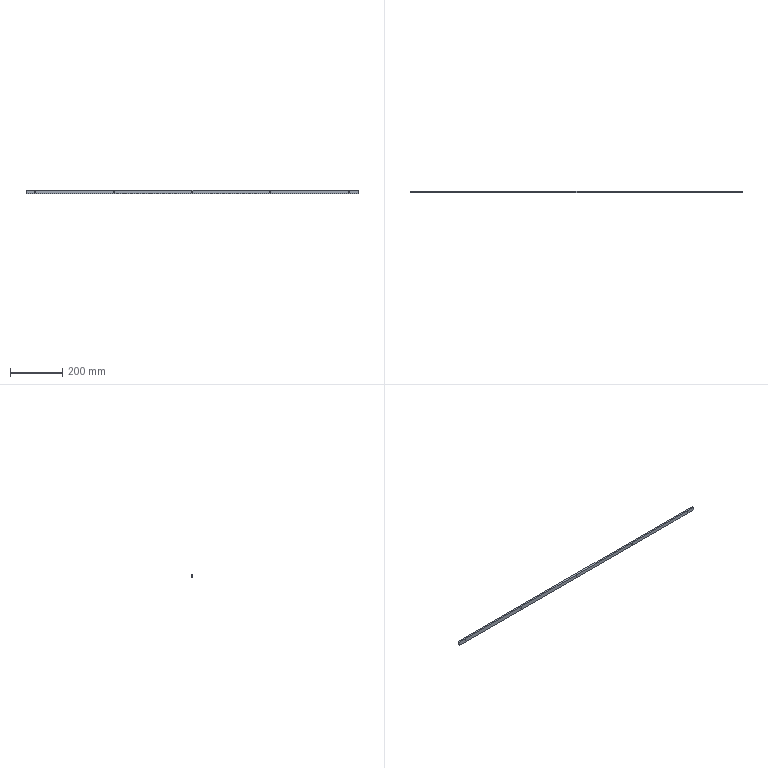Part | SolidWorks | features Chamfer 1, Extrusion 1, HoleWzd 1 | 1 solid | 33 faces | box 1270 x 6 x 15 mm | volume 113647 mm3 | cylinder 20 | plane 13 | commonest cylinder face diameters 3.4 x10 6 x10
STEP:
#1=CARTESIAN_POINT('',(-600.,-0.4,-3.));
#2=VERTEX_POINT('',#1);
#3=CARTESIAN_POINT('',(-600.,-0.4,3.));
#4=VERTEX_POINT('',#3);
#5=CARTESIAN_POINT('',(-600.,-0.4,0.));
#6=DIRECTION('',(0.,1.,0.));
#7=DIRECTION('',(0.,0.,1.));
#8=AXIS2_PLACEMENT_3D('',#5,#6,#7);
#9=CIRCLE('',#8,3.);
#10=EDGE_CURVE('',#2,#4,#9,.T.);
#11=ORIENTED_EDGE('',*,*,#10,.F.);
#12=CARTESIAN_POINT('',(-600.,3.,-3.));
#13=VERTEX_POINT('',#12);
#14=CARTESIAN_POINT('',(-600.,3.,-3.));
#15=DIRECTION('',(0.,1.,0.));
#16=VECTOR('',#15,1000.);
#17=LINE('',#14,#16);
#18=EDGE_CURVE('',#2,#13,#17,.T.);
#19=ORIENTED_EDGE('',*,*,#18,.T.);
#20=CARTESIAN_POINT('',(-600.,3.,3.));
#21=VERTEX_POINT('',#20);
#22=CARTESIAN_POINT('',(-600.,3.,0.));
#23=DIRECTION('',(0.,1.,0.));
#24=DIRECTION('',(0.,0.,1.));
#25=AXIS2_PLACEMENT_3D('',#22,#23,#24);
#26=CIRCLE('',#25,3.);
#27=EDGE_CURVE('',#13,#21,#26,.T.);
#28=ORIENTED_EDGE('',*,*,#27,.T.);
#29=CARTESIAN_POINT('',(-600.,3.,3.));
#30=DIRECTION('',(0.,1.,0.));
#31=VECTOR('',#30,1000.);
#32=LINE('',#29,#31);
#33=EDGE_CURVE('',#4,#21,#32,.T.);
#34=ORIENTED_EDGE('',*,*,#33,.F.);
#35=EDGE_LOOP('',(#11,#19,#28,#34));
#36=FACE_OUTER_BOUND('',#35,.T.);
#37=CARTESIAN_POINT('',(-600.,3.,0.));
#38=DIRECTION('',(0.,1.,0.));
#39=DIRECTION('',(0.,0.,1.));
#40=AXIS2_PLACEMENT_3D('',#37,#38,#39);
#41=CYLINDRICAL_SURFACE('',#40,3.);
#42=ADVANCED_FACE('',(#36),#41,.F.);
#43=CARTESIAN_POINT('',(-600.,-3.,-1.7));
#44=VERTEX_POINT('',#43);
#45=CARTESIAN_POINT('',(-600.,-3.,1.7));
#46=VERTEX_POINT('',#45);
#47=CARTESIAN_POINT('',(-600.,-3.,0.));
#48=DIRECTION('',(0.,1.,0.));
#49=DIRECTION('',(0.,0.,1.));
#50=AXIS2_PLACEMENT_3D('',#47,#48,#49);
#51=CIRCLE('',#50,1.7);
#52=EDGE_CURVE('',#44,#46,#51,.T.);
#53=ORIENTED_EDGE('',*,*,#52,.F.);
#54=CARTESIAN_POINT('',(-600.,-0.4,-1.7));
#55=VERTEX_POINT('',#54);
#56=CARTESIAN_POINT('',(-600.,3.,-1.7));
#57=DIRECTION('',(0.,1.,0.));
#58=VECTOR('',#57,1000.);
#59=LINE('',#56,#58);
#60=EDGE_CURVE('',#44,#55,#59,.T.);
#61=ORIENTED_EDGE('',*,*,#60,.T.);
#62=CARTESIAN_POINT('',(-600.,-0.4,1.7));
#63=VERTEX_POINT('',#62);
#64=CARTESIAN_POINT('',(-600.,-0.4,0.));
#65=DIRECTION('',(0.,1.,0.));
#66=DIRECTION('',(0.,0.,1.));
#67=AXIS2_PLACEMENT_3D('',#64,#65,#66);
#68=CIRCLE('',#67,1.7);
#69=EDGE_CURVE('',#55,#63,#68,.T.);
#70=ORIENTED_EDGE('',*,*,#69,.T.);
#71=CARTESIAN_POINT('',(-600.,3.,1.7));
#72=DIRECTION('',(0.,1.,0.));
#73=VECTOR('',#72,1000.);
#74=LINE('',#71,#73);
#75=EDGE_CURVE('',#46,#63,#74,.T.);
#76=ORIENTED_EDGE('',*,*,#75,.F.);
#77=EDGE_LOOP('',(#53,#61,#70,#76));
#78=FACE_OUTER_BOUND('',#77,.T.);
#79=CARTESIAN_POINT('',(-600.,3.,0.));
#80=DIRECTION('',(0.,1.,0.));
#81=DIRECTION('',(0.,0.,1.));
#82=AXIS2_PLACEMENT_3D('',#79,#80,#81);
#83=CYLINDRICAL_SURFACE('',#82,1.7);
#84=ADVANCED_FACE('',(#78),#83,.F.);
#85=CARTESIAN_POINT('',(-300.,-0.4,-3.));
#86=VERTEX_POINT('',#85);
#87=CARTESIAN_POINT('',(-300.,-0.4,3.));
#88=VERTEX_POINT('',#87);
#89=CARTESIAN_POINT('',(-300.,-0.4,0.));
#90=DIRECTION('',(0.,1.,0.));
#91=DIRECTION('',(0.,0.,1.));
#92=AXIS2_PLACEMENT_3D('',#89,#90,#91);
#93=CIRCLE('',#92,3.);
#94=EDGE_CURVE('',#86,#88,#93,.T.);
#95=ORIENTED_EDGE('',*,*,#94,.F.);
#96=CARTESIAN_POINT('',(-300.,3.,-3.));
#97=VERTEX_POINT('',#96);
#98=CARTESIAN_POINT('',(-300.,3.,-3.));
#99=DIRECTION('',(0.,1.,0.));
#100=VECTOR('',#99,1000.);
#101=LINE('',#98,#100);
#102=EDGE_CURVE('',#86,#97,#101,.T.);
#103=ORIENTED_EDGE('',*,*,#102,.T.);
#104=CARTESIAN_POINT('',(-300.,3.,3.));
#105=VERTEX_POINT('',#104);
#106=CARTESIAN_POINT('',(-300.,3.,0.));
#107=DIRECTION('',(0.,1.,0.));
#108=DIRECTION('',(0.,0.,1.));
#109=AXIS2_PLACEMENT_3D('',#106,#107,#108);
#110=CIRCLE('',#109,3.);
#111=EDGE_CURVE('',#97,#105,#110,.T.);
#112=ORIENTED_EDGE('',*,*,#111,.T.);
#113=CARTESIAN_POINT('',(-300.,3.,3.));
#114=DIRECTION('',(0.,1.,0.));
#115=VECTOR('',#114,1000.);
#116=LINE('',#113,#115);
#117=EDGE_CURVE('',#88,#105,#116,.T.);
#118=ORIENTED_EDGE('',*,*,#117,.F.);
#119=EDGE_LOOP('',(#95,#103,#112,#118));
#120=FACE_OUTER_BOUND('',#119,.T.);
#121=CARTESIAN_POINT('',(-300.,3.,0.));
#122=DIRECTION('',(0.,1.,0.));
#123=DIRECTION('',(0.,0.,1.));
#124=AXIS2_PLACEMENT_3D('',#121,#122,#123);
#125=CYLINDRICAL_SURFACE('',#124,3.);
#126=ADVANCED_FACE('',(#120),#125,.F.);
#127=CARTESIAN_POINT('',(-300.,-3.,-1.7));
#128=VERTEX_POINT('',#127);
#129=CARTESIAN_POINT('',(-300.,-3.,1.7));
#130=VERTEX_POINT('',#129);
#131=CARTESIAN_POINT('',(-300.,-3.,0.));
#132=DIRECTION('',(0.,1.,0.));
#133=DIRECTION('',(0.,0.,1.));
#134=AXIS2_PLACEMENT_3D('',#131,#132,#133);
#135=CIRCLE('',#134,1.7);
#136=EDGE_CURVE('',#128,#130,#135,.T.);
#137=ORIENTED_EDGE('',*,*,#136,.F.);
#138=CARTESIAN_POINT('',(-300.,-0.4,-1.7));
#139=VERTEX_POINT('',#138);
#140=CARTESIAN_POINT('',(-300.,3.,-1.7));
#141=DIRECTION('',(0.,1.,0.));
#142=VECTOR('',#141,1000.);
#143=LINE('',#140,#142);
#144=EDGE_CURVE('',#128,#139,#143,.T.);
#145=ORIENTED_EDGE('',*,*,#144,.T.);
#146=CARTESIAN_POINT('',(-300.,-0.4,1.7));
#147=VERTEX_POINT('',#146);
#148=CARTESIAN_POINT('',(-300.,-0.4,0.));
#149=DIRECTION('',(0.,1.,0.));
#150=DIRECTION('',(0.,0.,1.));
#151=AXIS2_PLACEMENT_3D('',#148,#149,#150);
#152=CIRCLE('',#151,1.7);
#153=EDGE_CURVE('',#139,#147,#152,.T.);
#154=ORIENTED_EDGE('',*,*,#153,.T.);
#155=CARTESIAN_POINT('',(-300.,3.,1.7));
#156=DIRECTION('',(0.,1.,0.));
#157=VECTOR('',#156,1000.);
#158=LINE('',#155,#157);
#159=EDGE_CURVE('',#130,#147,#158,.T.);
#160=ORIENTED_EDGE('',*,*,#159,.F.);
#161=EDGE_LOOP('',(#137,#145,#154,#160));
#162=FACE_OUTER_BOUND('',#161,.T.);
#163=CARTESIAN_POINT('',(-300.,3.,0.));
#164=DIRECTION('',(0.,1.,0.));
#165=DIRECTION('',(0.,0.,1.));
#166=AXIS2_PLACEMENT_3D('',#163,#164,#165);
#167=CYLINDRICAL_SURFACE('',#166,1.7);
#168=ADVANCED_FACE('',(#162),#167,.F.);
#169=CARTESIAN_POINT('',(0.,-0.4,-3.));
#170=VERTEX_POINT('',#169);
#171=CARTESIAN_POINT('',(0.,-0.4,3.));
#172=VERTEX_POINT('',#171);
#173=CARTESIAN_POINT('',(0.,-0.4,0.));
#174=DIRECTION('',(0.,1.,0.));
#175=DIRECTION('',(0.,0.,1.));
#176=AXIS2_PLACEMENT_3D('',#173,#174,#175);
#177=CIRCLE('',#176,3.);
#178=EDGE_CURVE('',#170,#172,#177,.T.);
#179=ORIENTED_EDGE('',*,*,#178,.F.);
#180=CARTESIAN_POINT('',(0.,3.,-3.));
#181=VERTEX_POINT('',#180);
#182=CARTESIAN_POINT('',(0.,3.,-3.));
#183=DIRECTION('',(0.,1.,0.));
#184=VECTOR('',#183,1000.);
#185=LINE('',#182,#184);
#186=EDGE_CURVE('',#170,#181,#185,.T.);
#187=ORIENTED_EDGE('',*,*,#186,.T.);
#188=CARTESIAN_POINT('',(0.,3.,3.));
#189=VERTEX_POINT('',#188);
#190=CARTESIAN_POINT('',(0.,3.,0.));
#191=DIRECTION('',(0.,1.,0.));
#192=DIRECTION('',(0.,0.,1.));
#193=AXIS2_PLACEMENT_3D('',#190,#191,#192);
#194=CIRCLE('',#193,3.);
#195=EDGE_CURVE('',#181,#189,#194,.T.);
#196=ORIENTED_EDGE('',*,*,#195,.T.);
#197=CARTESIAN_POINT('',(0.,3.,3.));
#198=DIRECTION('',(0.,1.,0.));
#199=VECTOR('',#198,1000.);
#200=LINE('',#197,#199);
#201=EDGE_CURVE('',#172,#189,#200,.T.);
#202=ORIENTED_EDGE('',*,*,#201,.F.);
#203=EDGE_LOOP('',(#179,#187,#196,#202));
#204=FACE_OUTER_BOUND('',#203,.T.);
#205=CARTESIAN_POINT('',(0.,3.,0.));
#206=DIRECTION('',(0.,1.,0.));
#207=DIRECTION('',(0.,0.,1.));
#208=AXIS2_PLACEMENT_3D('',#205,#206,#207);
#209=CYLINDRICAL_SURFACE('',#208,3.);
#210=ADVANCED_FACE('',(#204),#209,.F.);
#211=CARTESIAN_POINT('',(0.,-3.,-1.7));
#212=VERTEX_POINT('',#211);
#213=CARTESIAN_POINT('',(0.,-3.,1.7));
#214=VERTEX_POINT('',#213);
#215=CARTESIAN_POINT('',(0.,-3.,0.));
#216=DIRECTION('',(0.,1.,0.));
#217=DIRECTION('',(0.,0.,1.));
#218=AXIS2_PLACEMENT_3D('',#215,#216,#217);
#219=CIRCLE('',#218,1.7);
#220=EDGE_CURVE('',#212,#214,#219,.T.);
#221=ORIENTED_EDGE('',*,*,#220,.F.);
#222=CARTESIAN_POINT('',(0.,-0.4,-1.7));
#223=VERTEX_POINT('',#222);
#224=CARTESIAN_POINT('',(0.,3.,-1.7));
#225=DIRECTION('',(0.,1.,0.));
#226=VECTOR('',#225,1000.);
#227=LINE('',#224,#226);
#228=EDGE_CURVE('',#212,#223,#227,.T.);
#229=ORIENTED_EDGE('',*,*,#228,.T.);
#230=CARTESIAN_POINT('',(0.,-0.4,1.7));
#231=VERTEX_POINT('',#230);
#232=CARTESIAN_POINT('',(0.,-0.4,0.));
#233=DIRECTION('',(0.,1.,0.));
#234=DIRECTION('',(0.,0.,1.));
#235=AXIS2_PLACEMENT_3D('',#232,#233,#234);
#236=CIRCLE('',#235,1.7);
#237=EDGE_CURVE('',#223,#231,#236,.T.);
#238=ORIENTED_EDGE('',*,*,#237,.T.);
#239=CARTESIAN_POINT('',(0.,3.,1.7));
#240=DIRECTION('',(0.,1.,0.));
#241=VECTOR('',#240,1000.);
#242=LINE('',#239,#241);
#243=EDGE_CURVE('',#214,#231,#242,.T.);
#244=ORIENTED_EDGE('',*,*,#243,.F.);
#245=EDGE_LOOP('',(#221,#229,#238,#244));
#246=FACE_OUTER_BOUND('',#245,.T.);
#247=CARTESIAN_POINT('',(0.,3.,0.));
#248=DIRECTION('',(0.,1.,0.));
#249=DIRECTION('',(0.,0.,1.));
#250=AXIS2_PLACEMENT_3D('',#247,#248,#249);
#251=CYLINDRICAL_SURFACE('',#250,1.7);
#252=ADVANCED_FACE('',(#246),#251,.F.);
#253=CARTESIAN_POINT('',(300.,-0.4,-3.));
#254=VERTEX_POINT('',#253);
#255=CARTESIAN_POINT('',(300.,-0.4,3.));
#256=VERTEX_POINT('',#255);
#257=CARTESIAN_POINT('',(300.,-0.4,0.));
#258=DIRECTION('',(0.,1.,0.));
#259=DIRECTION('',(0.,0.,1.));
#260=AXIS2_PLACEMENT_3D('',#257,#258,#259);
#261=CIRCLE('',#260,3.);
#262=EDGE_CURVE('',#254,#256,#261,.T.);
#263=ORIENTED_EDGE('',*,*,#262,.F.);
#264=CARTESIAN_POINT('',(300.,3.,-3.));
#265=VERTEX_POINT('',#264);
#266=CARTESIAN_POINT('',(300.,3.,-3.));
#267=DIRECTION('',(0.,1.,0.));
#268=VECTOR('',#267,1000.);
#269=LINE('',#266,#268);
#270=EDGE_CURVE('',#254,#265,#269,.T.);
#271=ORIENTED_EDGE('',*,*,#270,.T.);
#272=CARTESIAN_POINT('',(300.,3.,3.));
#273=VERTEX_POINT('',#272);
#274=CARTESIAN_POINT('',(300.,3.,0.));
#275=DIRECTION('',(0.,1.,0.));
#276=DIRECTION('',(0.,0.,1.));
#277=AXIS2_PLACEMENT_3D('',#274,#275,#276);
#278=CIRCLE('',#277,3.);
#279=EDGE_CURVE('',#265,#273,#278,.T.);
#280=ORIENTED_EDGE('',*,*,#279,.T.);
#281=CARTESIAN_POINT('',(300.,3.,3.));
#282=DIRECTION('',(0.,1.,0.));
#283=VECTOR('',#282,1000.);
#284=LINE('',#281,#283);
#285=EDGE_CURVE('',#256,#273,#284,.T.);
#286=ORIENTED_EDGE('',*,*,#285,.F.);
#287=EDGE_LOOP('',(#263,#271,#280,#286));
#288=FACE_OUTER_BOUND('',#287,.T.);
#289=CARTESIAN_POINT('',(300.,3.,0.));
#290=DIRECTION('',(0.,1.,0.));
#291=DIRECTION('',(0.,0.,1.));
#292=AXIS2_PLACEMENT_3D('',#289,#290,#291);
#293=CYLINDRICAL_SURFACE('',#292,3.);
#294=ADVANCED_FACE('',(#288),#293,.F.);
#295=CARTESIAN_POINT('',(300.,-3.,-1.7));
#296=VERTEX_POINT('',#295);
#297=CARTESIAN_POINT('',(300.,-3.,1.7));
#298=VERTEX_POINT('',#297);
#299=CARTESIAN_POINT('',(300.,-3.,0.));
#300=DIRECTION('',(0.,1.,0.));
#301=DIRECTION('',(0.,0.,1.));
#302=AXIS2_PLACEMENT_3D('',#299,#300,#301);
#303=CIRCLE('',#302,1.7);
#304=EDGE_CURVE('',#296,#298,#303,.T.);
#305=ORIENTED_EDGE('',*,*,#304,.F.);
#306=CARTESIAN_POINT('',(300.,-0.4,-1.7));
#307=VERTEX_POINT('',#306);
#308=CARTESIAN_POINT('',(300.,3.,-1.7));
#309=DIRECTION('',(0.,1.,0.));
#310=VECTOR('',#309,1000.);
#311=LINE('',#308,#310);
#312=EDGE_CURVE('',#296,#307,#311,.T.);
#313=ORIENTED_EDGE('',*,*,#312,.T.);
#314=CARTESIAN_POINT('',(300.,-0.4,1.7));
#315=VERTEX_POINT('',#314);
#316=CARTESIAN_POINT('',(300.,-0.4,0.));
#317=DIRECTION('',(0.,1.,0.));
#318=DIRECTION('',(0.,0.,1.));
#319=AXIS2_PLACEMENT_3D('',#316,#317,#318);
#320=CIRCLE('',#319,1.7);
#321=EDGE_CURVE('',#307,#315,#320,.T.);
#322=ORIENTED_EDGE('',*,*,#321,.T.);
#323=CARTESIAN_POINT('',(300.,3.,1.7));
#324=DIRECTION('',(0.,1.,0.));
#325=VECTOR('',#324,1000.);
#326=LINE('',#323,#325);
#327=EDGE_CURVE('',#298,#315,#326,.T.);
#328=ORIENTED_EDGE('',*,*,#327,.F.);
#329=EDGE_LOOP('',(#305,#313,#322,#328));
#330=FACE_OUTER_BOUND('',#329,.T.);
#331=CARTESIAN_POINT('',(300.,3.,0.));
#332=DIRECTION('',(0.,1.,0.));
#333=DIRECTION('',(0.,0.,1.));
#334=AXIS2_PLACEMENT_3D('',#331,#332,#333);
#335=CYLINDRICAL_SURFACE('',#334,1.7);
#336=ADVANCED_FACE('',(#330),#335,.F.);
#337=CARTESIAN_POINT('',(600.,-0.4,-3.));
#338=VERTEX_POINT('',#337);
#339=CARTESIAN_POINT('',(600.,-0.4,3.));
#340=VERTEX_POINT('',#339);
#341=CARTESIAN_POINT('',(600.,-0.4,0.));
#342=DIRECTION('',(0.,1.,0.));
#343=DIRECTION('',(0.,0.,1.));
#344=AXIS2_PLACEMENT_3D('',#341,#342,#343);
#345=CIRCLE('',#344,3.);
#346=EDGE_CURVE('',#338,#340,#345,.T.);
#347=ORIENTED_EDGE('',*,*,#346,.F.);
#348=CARTESIAN_POINT('',(600.,3.,-3.));
#349=VERTEX_POINT('',#348);
#350=CARTESIAN_POINT('',(600.,3.,-3.));
#351=DIRECTION('',(0.,1.,0.));
#352=VECTOR('',#351,1000.);
#353=LINE('',#350,#352);
#354=EDGE_CURVE('',#338,#349,#353,.T.);
#355=ORIENTED_EDGE('',*,*,#354,.T.);
#356=CARTESIAN_POINT('',(600.,3.,3.));
#357=VERTEX_POINT('',#356);
#358=CARTESIAN_POINT('',(600.,3.,0.));
#359=DIRECTION('',(0.,1.,0.));
#360=DIRECTION('',(0.,0.,1.));
#361=AXIS2_PLACEMENT_3D('',#358,#359,#360);
#362=CIRCLE('',#361,3.);
#363=EDGE_CURVE('',#349,#357,#362,.T.);
#364=ORIENTED_EDGE('',*,*,#363,.T.);
#365=CARTESIAN_POINT('',(600.,3.,3.));
#366=DIRECTION('',(0.,1.,0.));
#367=VECTOR('',#366,1000.);
#368=LINE('',#365,#367);
#369=EDGE_CURVE('',#340,#357,#368,.T.);
#370=ORIENTED_EDGE('',*,*,#369,.F.);
#371=EDGE_LOOP('',(#347,#355,#364,#370));
#372=FACE_OUTER_BOUND('',#371,.T.);
#373=CARTESIAN_POINT('',(600.,3.,0.));
#374=DIRECTION('',(0.,1.,0.));
#375=DIRECTION('',(0.,0.,1.));
#376=AXIS2_PLACEMENT_3D('',#373,#374,#375);
#377=CYLINDRICAL_SURFACE('',#376,3.);
#378=ADVANCED_FACE('',(#372),#377,.F.);
#379=CARTESIAN_POINT('',(600.,-3.,-1.7));
#380=VERTEX_POINT('',#379);
#381=CARTESIAN_POINT('',(600.,-3.,1.7));
#382=VERTEX_POINT('',#381);
#383=CARTESIAN_POINT('',(600.,-3.,0.));
#384=DIRECTION('',(0.,1.,0.));
#385=DIRECTION('',(0.,0.,1.));
#386=AXIS2_PLACEMENT_3D('',#383,#384,#385);
#387=CIRCLE('',#386,1.7);
#388=EDGE_CURVE('',#380,#382,#387,.T.);
#389=ORIENTED_EDGE('',*,*,#388,.F.);
#390=CARTESIAN_POINT('',(600.,-0.4,-1.7));
#391=VERTEX_POINT('',#390);
#392=CARTESIAN_POINT('',(600.,3.,-1.7));
#393=DIRECTION('',(0.,1.,0.));
#394=VECTOR('',#393,1000.);
#395=LINE('',#392,#394);
#396=EDGE_CURVE('',#380,#391,#395,.T.);
#397=ORIENTED_EDGE('',*,*,#396,.T.);
#398=CARTESIAN_POINT('',(600.,-0.4,1.7));
#399=VERTEX_POINT('',#398);
#400=CARTESIAN_POINT('',(600.,-0.4,0.));
#401=DIRECTION('',(0.,1.,0.));
#402=DIRECTION('',(0.,0.,1.));
#403=AXIS2_PLACEMENT_3D('',#400,#401,#402);
#404=CIRCLE('',#403,1.7);
#405=EDGE_CURVE('',#391,#399,#404,.T.);
#406=ORIENTED_EDGE('',*,*,#405,.T.);
#407=CARTESIAN_POINT('',(600.,3.,1.7));
#408=DIRECTION('',(0.,1.,0.));
#409=VECTOR('',#408,1000.);
#410=LINE('',#407,#409);
#411=EDGE_CURVE('',#382,#399,#410,.T.);
#412=ORIENTED_EDGE('',*,*,#411,.F.);
#413=EDGE_LOOP('',(#389,#397,#406,#412));
#414=FACE_OUTER_BOUND('',#413,.T.);
#415=CARTESIAN_POINT('',(600.,3.,0.));
#416=DIRECTION('',(0.,1.,0.));
#417=DIRECTION('',(0.,0.,1.));
#418=AXIS2_PLACEMENT_3D('',#415,#416,#417);
#419=CYLINDRICAL_SURFACE('',#418,1.7);
#420=ADVANCED_FACE('',(#414),#419,.F.);
#421=CARTESIAN_POINT('',(635.,3.,4.5));
#422=VERTEX_POINT('',#421);
#423=CARTESIAN_POINT('',(635.,3.,-7.5));
#424=VERTEX_POINT('',#423);
#425=CARTESIAN_POINT('',(635.,3.,7.5));
#426=DIRECTION('',(0.,0.,-1.));
#427=VECTOR('',#426,1000.);
#428=LINE('',#425,#427);
#429=EDGE_CURVE('',#422,#424,#428,.T.);
#430=ORIENTED_EDGE('',*,*,#429,.F.);
#431=CARTESIAN_POINT('',(635.,-3.,4.5));
#432=VERTEX_POINT('',#431);
#433=CARTESIAN_POINT('',(635.,3.,4.5));
#434=DIRECTION('',(0.,-1.,0.));
#435=VECTOR('',#434,1000.);
#436=LINE('',#433,#435);
#437=EDGE_CURVE('',#422,#432,#436,.T.);
#438=ORIENTED_EDGE('',*,*,#437,.T.);
#439=CARTESIAN_POINT('',(635.,-3.,-7.5));
#440=VERTEX_POINT('',#439);
#441=CARTESIAN_POINT('',(635.,-3.,7.5));
#442=DIRECTION('',(0.,0.,-1.));
#443=VECTOR('',#442,1000.);
#444=LINE('',#441,#443);
#445=EDGE_CURVE('',#432,#440,#444,.T.);
#446=ORIENTED_EDGE('',*,*,#445,.T.);
#447=CARTESIAN_POINT('',(635.,3.,-7.5));
#448=DIRECTION('',(0.,-1.,0.));
#449=VECTOR('',#448,1000.);
#450=LINE('',#447,#449);
#451=EDGE_CURVE('',#424,#440,#450,.T.);
#452=ORIENTED_EDGE('',*,*,#451,.F.);
#453=EDGE_LOOP('',(#430,#438,#446,#452));
#454=FACE_OUTER_BOUND('',#453,.T.);
#455=CARTESIAN_POINT('',(635.,3.,7.5));
#456=DIRECTION('',(-1.,0.,0.));
#457=DIRECTION('',(0.,0.,1.));
#458=AXIS2_PLACEMENT_3D('',#455,#456,#457);
#459=PLANE('',#458);
#460=ADVANCED_FACE('',(#454),#459,.F.);
#461=CARTESIAN_POINT('',(-635.,-3.,-7.5));
#462=VERTEX_POINT('',#461);
#463=CARTESIAN_POINT('',(-635.,-3.,-7.5));
#464=DIRECTION('',(-1.,0.,0.));
#465=VECTOR('',#464,1000.);
#466=LINE('',#463,#465);
#467=EDGE_CURVE('',#440,#462,#466,.T.);
#468=ORIENTED_EDGE('',*,*,#467,.T.);
#469=CARTESIAN_POINT('',(-635.,3.,-7.5));
#470=VERTEX_POINT('',#469);
#471=CARTESIAN_POINT('',(-635.,3.,-7.5));
#472=DIRECTION('',(0.,-1.,0.));
#473=VECTOR('',#472,1000.);
#474=LINE('',#471,#473);
#475=EDGE_CURVE('',#470,#462,#474,.T.);
#476=ORIENTED_EDGE('',*,*,#475,.F.);
#477=CARTESIAN_POINT('',(-635.,3.,-7.5));
#478=DIRECTION('',(-1.,0.,0.));
#479=VECTOR('',#478,1000.);
#480=LINE('',#477,#479);
#481=EDGE_CURVE('',#424,#470,#480,.T.);
#482=ORIENTED_EDGE('',*,*,#481,.F.);
#483=ORIENTED_EDGE('',*,*,#451,.T.);
#484=EDGE_LOOP('',(#468,#476,#482,#483));
#485=FACE_OUTER_BOUND('',#484,.T.);
#486=CARTESIAN_POINT('',(-635.,3.,-7.5));
#487=DIRECTION('',(0.,0.,1.));
#488=DIRECTION('',(1.,0.,0.));
#489=AXIS2_PLACEMENT_3D('',#486,#487,#488);
#490=PLANE('',#489);
#491=ADVANCED_FACE('',(#485),#490,.F.);
#492=CARTESIAN_POINT('',(-635.,-3.,4.5));
#493=VERTEX_POINT('',#492);
#494=CARTESIAN_POINT('',(-635.,-3.,7.5));
#495=DIRECTION('',(0.,0.,1.));
#496=VECTOR('',#495,1000.);
#497=LINE('',#494,#496);
#498=EDGE_CURVE('',#462,#493,#497,.T.);
#499=ORIENTED_EDGE('',*,*,#498,.T.);
#500=CARTESIAN_POINT('',(-635.,3.,4.5));
#501=VERTEX_POINT('',#500);
#502=CARTESIAN_POINT('',(-635.,3.,4.5));
#503=DIRECTION('',(0.,1.,0.));
#504=VECTOR('',#503,1000.);
#505=LINE('',#502,#504);
#506=EDGE_CURVE('',#493,#501,#505,.T.);
#507=ORIENTED_EDGE('',*,*,#506,.T.);
#508=CARTESIAN_POINT('',(-635.,3.,7.5));
#509=DIRECTION('',(0.,0.,1.));
#510=VECTOR('',#509,1000.);
#511=LINE('',#508,#510);
#512=EDGE_CURVE('',#470,#501,#511,.T.);
#513=ORIENTED_EDGE('',*,*,#512,.F.);
#514=ORIENTED_EDGE('',*,*,#475,.T.);
#515=EDGE_LOOP('',(#499,#507,#513,#514));
#516=FACE_OUTER_BOUND('',#515,.T.);
#517=CARTESIAN_POINT('',(-635.,3.,7.5));
#518=DIRECTION('',(1.,0.,0.));
#519=DIRECTION('',(0.,0.,-1.));
#520=AXIS2_PLACEMENT_3D('',#517,#518,#519);
#521=PLANE('',#520);
#522=ADVANCED_FACE('',(#516),#521,.F.);
#523=CARTESIAN_POINT('',(-632.,3.,7.5));
#524=VERTEX_POINT('',#523);
#525=CARTESIAN_POINT('',(632.,3.,7.5));
#526=VERTEX_POINT('',#525);
#527=CARTESIAN_POINT('',(-635.,3.,7.5));
#528=DIRECTION('',(1.,0.,0.));
#529=VECTOR('',#528,1000.);
#530=LINE('',#527,#529);
#531=EDGE_CURVE('',#524,#526,#530,.T.);
#532=ORIENTED_EDGE('',*,*,#531,.F.);
#533=CARTESIAN_POINT('',(-632.,-3.,7.5));
#534=VERTEX_POINT('',#533);
#535=CARTESIAN_POINT('',(-632.,3.,7.5));
#536=DIRECTION('',(0.,-1.,0.));
#537=VECTOR('',#536,1000.);
#538=LINE('',#535,#537);
#539=EDGE_CURVE('',#524,#534,#538,.T.);
#540=ORIENTED_EDGE('',*,*,#539,.T.);
#541=CARTESIAN_POINT('',(632.,-3.,7.5));
#542=VERTEX_POINT('',#541);
#543=CARTESIAN_POINT('',(-635.,-3.,7.5));
#544=DIRECTION('',(1.,0.,0.));
#545=VECTOR('',#544,1000.);
#546=LINE('',#543,#545);
#547=EDGE_CURVE('',#534,#542,#546,.T.);
#548=ORIENTED_EDGE('',*,*,#547,.T.);
#549=CARTESIAN_POINT('',(632.,3.,7.5));
#550=DIRECTION('',(0.,1.,0.));
#551=VECTOR('',#550,1000.);
#552=LINE('',#549,#551);
#553=EDGE_CURVE('',#542,#526,#552,.T.);
#554=ORIENTED_EDGE('',*,*,#553,.T.);
#555=EDGE_LOOP('',(#532,#540,#548,#554));
#556=FACE_OUTER_BOUND('',#555,.T.);
#557=CARTESIAN_POINT('',(-635.,3.,7.5));
#558=DIRECTION('',(0.,0.,-1.));
#559=DIRECTION('',(-1.,0.,0.));
#560=AXIS2_PLACEMENT_3D('',#557,#558,#559);
#561=PLANE('',#560);
#562=ADVANCED_FACE('',(#556),#561,.F.);
#563=CARTESIAN_POINT('',(-600.,3.,0.));
#564=DIRECTION('',(0.,1.,0.));
#565=DIRECTION('',(0.,0.,1.));
#566=AXIS2_PLACEMENT_3D('',#563,#564,#565);
#567=CIRCLE('',#566,3.);
#568=EDGE_CURVE('',#21,#13,#567,.T.);
#569=ORIENTED_EDGE('',*,*,#568,.F.);
#570=ORIENTED_EDGE('',*,*,#27,.F.);
#571=EDGE_LOOP('',(#569,#570));
#572=FACE_BOUND('',#571,.T.);
#573=CARTESIAN_POINT('',(-300.,3.,0.));
#574=DIRECTION('',(0.,1.,0.));
#575=DIRECTION('',(0.,0.,1.));
#576=AXIS2_PLACEMENT_3D('',#573,#574,#575);
#577=CIRCLE('',#576,3.);
#578=EDGE_CURVE('',#105,#97,#577,.T.);
#579=ORIENTED_EDGE('',*,*,#578,.F.);
#580=ORIENTED_EDGE('',*,*,#111,.F.);
#581=EDGE_LOOP('',(#579,#580));
#582=FACE_BOUND('',#581,.T.);
#583=CARTESIAN_POINT('',(0.,3.,0.));
#584=DIRECTION('',(0.,1.,0.));
#585=DIRECTION('',(0.,0.,1.));
#586=AXIS2_PLACEMENT_3D('',#583,#584,#585);
#587=CIRCLE('',#586,3.);
#588=EDGE_CURVE('',#189,#181,#587,.T.);
#589=ORIENTED_EDGE('',*,*,#588,.F.);
#590=ORIENTED_EDGE('',*,*,#195,.F.);
#591=EDGE_LOOP('',(#589,#590));
#592=FACE_BOUND('',#591,.T.);
#593=CARTESIAN_POINT('',(300.,3.,0.));
#594=DIRECTION('',(0.,1.,0.));
#595=DIRECTION('',(0.,0.,1.));
#596=AXIS2_PLACEMENT_3D('',#593,#594,#595);
#597=CIRCLE('',#596,3.);
#598=EDGE_CURVE('',#273,#265,#597,.T.);
#599=ORIENTED_EDGE('',*,*,#598,.F.);
#600=ORIENTED_EDGE('',*,*,#279,.F.);
#601=EDGE_LOOP('',(#599,#600));
#602=FACE_BOUND('',#601,.T.);
#603=CARTESIAN_POINT('',(600.,3.,0.));
#604=DIRECTION('',(0.,1.,0.));
#605=DIRECTION('',(0.,0.,1.));
#606=AXIS2_PLACEMENT_3D('',#603,#604,#605);
#607=CIRCLE('',#606,3.);
#608=EDGE_CURVE('',#357,#349,#607,.T.);
#609=ORIENTED_EDGE('',*,*,#608,.F.);
#610=ORIENTED_EDGE('',*,*,#363,.F.);
#611=EDGE_LOOP('',(#609,#610));
#612=FACE_BOUND('',#611,.T.);
#613=ORIENTED_EDGE('',*,*,#512,.T.);
#614=CARTESIAN_POINT('',(-632.,3.,7.5));
#615=DIRECTION('',(0.7071,0.,0.7071));
#616=VECTOR('',#615,1000.);
#617=LINE('',#614,#616);
#618=EDGE_CURVE('',#501,#524,#617,.T.);
#619=ORIENTED_EDGE('',*,*,#618,.T.);
#620=ORIENTED_EDGE('',*,*,#531,.T.);
#621=CARTESIAN_POINT('',(635.,3.,4.5));
#622=DIRECTION('',(0.7071,0.,-0.7071));
#623=VECTOR('',#622,1000.);
#624=LINE('',#621,#623);
#625=EDGE_CURVE('',#526,#422,#624,.T.);
#626=ORIENTED_EDGE('',*,*,#625,.T.);
#627=ORIENTED_EDGE('',*,*,#429,.T.);
#628=ORIENTED_EDGE('',*,*,#481,.T.);
#629=EDGE_LOOP('',(#613,#619,#620,#626,#627,#628));
#630=FACE_OUTER_BOUND('',#629,.T.);
#631=CARTESIAN_POINT('',(0.,3.,0.));
#632=DIRECTION('',(0.,-1.,0.));
#633=DIRECTION('',(0.,0.,-1.));
#634=AXIS2_PLACEMENT_3D('',#631,#632,#633);
#635=PLANE('',#634);
#636=ADVANCED_FACE('',(#572,#582,#592,#602,#612,#630),#635,.F.);
#637=CARTESIAN_POINT('',(-600.,-3.,0.));
#638=DIRECTION('',(0.,1.,0.));
#639=DIRECTION('',(0.,0.,1.));
#640=AXIS2_PLACEMENT_3D('',#637,#638,#639);
#641=CIRCLE('',#640,1.7);
#642=EDGE_CURVE('',#46,#44,#641,.T.);
#643=ORIENTED_EDGE('',*,*,#642,.T.);
#644=ORIENTED_EDGE('',*,*,#52,.T.);
#645=EDGE_LOOP('',(#643,#644));
#646=FACE_BOUND('',#645,.T.);
#647=CARTESIAN_POINT('',(-300.,-3.,0.));
#648=DIRECTION('',(0.,1.,0.));
#649=DIRECTION('',(0.,0.,1.));
#650=AXIS2_PLACEMENT_3D('',#647,#648,#649);
#651=CIRCLE('',#650,1.7);
#652=EDGE_CURVE('',#130,#128,#651,.T.);
#653=ORIENTED_EDGE('',*,*,#652,.T.);
#654=ORIENTED_EDGE('',*,*,#136,.T.);
#655=EDGE_LOOP('',(#653,#654));
#656=FACE_BOUND('',#655,.T.);
#657=CARTESIAN_POINT('',(0.,-3.,0.));
#658=DIRECTION('',(0.,1.,0.));
#659=DIRECTION('',(0.,0.,1.));
#660=AXIS2_PLACEMENT_3D('',#657,#658,#659);
#661=CIRCLE('',#660,1.7);
#662=EDGE_CURVE('',#214,#212,#661,.T.);
#663=ORIENTED_EDGE('',*,*,#662,.T.);
#664=ORIENTED_EDGE('',*,*,#220,.T.);
#665=EDGE_LOOP('',(#663,#664));
#666=FACE_BOUND('',#665,.T.);
#667=CARTESIAN_POINT('',(300.,-3.,0.));
#668=DIRECTION('',(0.,1.,0.));
#669=DIRECTION('',(0.,0.,1.));
#670=AXIS2_PLACEMENT_3D('',#667,#668,#669);
#671=CIRCLE('',#670,1.7);
#672=EDGE_CURVE('',#298,#296,#671,.T.);
#673=ORIENTED_EDGE('',*,*,#672,.T.);
#674=ORIENTED_EDGE('',*,*,#304,.T.);
#675=EDGE_LOOP('',(#673,#674));
#676=FACE_BOUND('',#675,.T.);
#677=CARTESIAN_POINT('',(600.,-3.,0.));
#678=DIRECTION('',(0.,1.,0.));
#679=DIRECTION('',(0.,0.,1.));
#680=AXIS2_PLACEMENT_3D('',#677,#678,#679);
#681=CIRCLE('',#680,1.7);
#682=EDGE_CURVE('',#382,#380,#681,.T.);
#683=ORIENTED_EDGE('',*,*,#682,.T.);
#684=ORIENTED_EDGE('',*,*,#388,.T.);
#685=EDGE_LOOP('',(#683,#684));
#686=FACE_BOUND('',#685,.T.);
#687=ORIENTED_EDGE('',*,*,#547,.F.);
#688=CARTESIAN_POINT('',(-319.75,-3.,319.75));
#689=DIRECTION('',(-0.7071,0.,-0.7071));
#690=VECTOR('',#689,1000.);
#691=LINE('',#688,#690);
#692=EDGE_CURVE('',#534,#493,#691,.T.);
#693=ORIENTED_EDGE('',*,*,#692,.T.);
#694=ORIENTED_EDGE('',*,*,#498,.F.);
#695=ORIENTED_EDGE('',*,*,#467,.F.);
#696=ORIENTED_EDGE('',*,*,#445,.F.);
#697=CARTESIAN_POINT('',(319.75,-3.,319.75));
#698=DIRECTION('',(-0.7071,0.,0.7071));
#699=VECTOR('',#698,1000.);
#700=LINE('',#697,#699);
#701=EDGE_CURVE('',#432,#542,#700,.T.);
#702=ORIENTED_EDGE('',*,*,#701,.T.);
#703=EDGE_LOOP('',(#687,#693,#694,#695,#696,#702));
#704=FACE_OUTER_BOUND('',#703,.T.);
#705=CARTESIAN_POINT('',(0.,-3.,0.));
#706=DIRECTION('',(0.,-1.,0.));
#707=DIRECTION('',(0.,0.,-1.));
#708=AXIS2_PLACEMENT_3D('',#705,#706,#707);
#709=PLANE('',#708);
#710=ADVANCED_FACE('',(#646,#656,#666,#676,#686,#704),#709,.T.);
#711=ORIENTED_EDGE('',*,*,#618,.F.);
#712=ORIENTED_EDGE('',*,*,#506,.F.);
#713=ORIENTED_EDGE('',*,*,#692,.F.);
#714=ORIENTED_EDGE('',*,*,#539,.F.);
#715=EDGE_LOOP('',(#711,#712,#713,#714));
#716=FACE_OUTER_BOUND('',#715,.T.);
#717=CARTESIAN_POINT('',(-632.,3.,7.5));
#718=DIRECTION('',(0.7071,0.,-0.7071));
#719=DIRECTION('',(0.,-1.,0.));
#720=AXIS2_PLACEMENT_3D('',#717,#718,#719);
#721=PLANE('',#720);
#722=ADVANCED_FACE('',(#716),#721,.F.);
#723=ORIENTED_EDGE('',*,*,#625,.F.);
#724=ORIENTED_EDGE('',*,*,#553,.F.);
#725=ORIENTED_EDGE('',*,*,#701,.F.);
#726=ORIENTED_EDGE('',*,*,#437,.F.);
#727=EDGE_LOOP('',(#723,#724,#725,#726));
#728=FACE_OUTER_BOUND('',#727,.T.);
#729=CARTESIAN_POINT('',(635.,3.,4.5));
#730=DIRECTION('',(-0.7071,0.,-0.7071));
#731=DIRECTION('',(0.,-1.,0.));
#732=AXIS2_PLACEMENT_3D('',#729,#730,#731);
#733=PLANE('',#732);
#734=ADVANCED_FACE('',(#728),#733,.F.);
#735=ORIENTED_EDGE('',*,*,#396,.F.);
#736=ORIENTED_EDGE('',*,*,#682,.F.);
#737=ORIENTED_EDGE('',*,*,#411,.T.);
#738=CARTESIAN_POINT('',(600.,-0.4,0.));
#739=DIRECTION('',(0.,1.,0.));
#740=DIRECTION('',(0.,0.,1.));
#741=AXIS2_PLACEMENT_3D('',#738,#739,#740);
#742=CIRCLE('',#741,1.7);
#743=EDGE_CURVE('',#399,#391,#742,.T.);
#744=ORIENTED_EDGE('',*,*,#743,.T.);
#745=EDGE_LOOP('',(#735,#736,#737,#744));
#746=FACE_OUTER_BOUND('',#745,.T.);
#747=CARTESIAN_POINT('',(600.,3.,0.));
#748=DIRECTION('',(0.,1.,0.));
#749=DIRECTION('',(0.,0.,1.));
#750=AXIS2_PLACEMENT_3D('',#747,#748,#749);
#751=CYLINDRICAL_SURFACE('',#750,1.7);
#752=ADVANCED_FACE('',(#746),#751,.F.);
#753=ORIENTED_EDGE('',*,*,#743,.F.);
#754=ORIENTED_EDGE('',*,*,#405,.F.);
#755=EDGE_LOOP('',(#753,#754));
#756=FACE_BOUND('',#755,.T.);
#757=CARTESIAN_POINT('',(600.,-0.4,0.));
#758=DIRECTION('',(0.,1.,0.));
#759=DIRECTION('',(0.,0.,1.));
#760=AXIS2_PLACEMENT_3D('',#757,#758,#759);
#761=CIRCLE('',#760,3.);
#762=EDGE_CURVE('',#340,#338,#761,.T.);
#763=ORIENTED_EDGE('',*,*,#762,.T.);
#764=ORIENTED_EDGE('',*,*,#346,.T.);
#765=EDGE_LOOP('',(#763,#764));
#766=FACE_OUTER_BOUND('',#765,.T.);
#767=CARTESIAN_POINT('',(601.7,-0.4,0.));
#768=DIRECTION('',(0.,-1.,0.));
#769=DIRECTION('',(0.,0.,-1.));
#770=AXIS2_PLACEMENT_3D('',#767,#768,#769);
#771=PLANE('',#770);
#772=ADVANCED_FACE('',(#756,#766),#771,.F.);
#773=ORIENTED_EDGE('',*,*,#354,.F.);
#774=ORIENTED_EDGE('',*,*,#762,.F.);
#775=ORIENTED_EDGE('',*,*,#369,.T.);
#776=ORIENTED_EDGE('',*,*,#608,.T.);
#777=EDGE_LOOP('',(#773,#774,#775,#776));
#778=FACE_OUTER_BOUND('',#777,.T.);
#779=CARTESIAN_POINT('',(600.,3.,0.));
#780=DIRECTION('',(0.,1.,0.));
#781=DIRECTION('',(0.,0.,1.));
#782=AXIS2_PLACEMENT_3D('',#779,#780,#781);
#783=CYLINDRICAL_SURFACE('',#782,3.);
#784=ADVANCED_FACE('',(#778),#783,.F.);
#785=ORIENTED_EDGE('',*,*,#312,.F.);
#786=ORIENTED_EDGE('',*,*,#672,.F.);
#787=ORIENTED_EDGE('',*,*,#327,.T.);
#788=CARTESIAN_POINT('',(300.,-0.4,0.));
#789=DIRECTION('',(0.,1.,0.));
#790=DIRECTION('',(0.,0.,1.));
#791=AXIS2_PLACEMENT_3D('',#788,#789,#790);
#792=CIRCLE('',#791,1.7);
#793=EDGE_CURVE('',#315,#307,#792,.T.);
#794=ORIENTED_EDGE('',*,*,#793,.T.);
#795=EDGE_LOOP('',(#785,#786,#787,#794));
#796=FACE_OUTER_BOUND('',#795,.T.);
#797=CARTESIAN_POINT('',(300.,3.,0.));
#798=DIRECTION('',(0.,1.,0.));
#799=DIRECTION('',(0.,0.,1.));
#800=AXIS2_PLACEMENT_3D('',#797,#798,#799);
#801=CYLINDRICAL_SURFACE('',#800,1.7);
#802=ADVANCED_FACE('',(#796),#801,.F.);
#803=ORIENTED_EDGE('',*,*,#793,.F.);
#804=ORIENTED_EDGE('',*,*,#321,.F.);
#805=EDGE_LOOP('',(#803,#804));
#806=FACE_BOUND('',#805,.T.);
#807=CARTESIAN_POINT('',(300.,-0.4,0.));
#808=DIRECTION('',(0.,1.,0.));
#809=DIRECTION('',(0.,0.,1.));
#810=AXIS2_PLACEMENT_3D('',#807,#808,#809);
#811=CIRCLE('',#810,3.);
#812=EDGE_CURVE('',#256,#254,#811,.T.);
#813=ORIENTED_EDGE('',*,*,#812,.T.);
#814=ORIENTED_EDGE('',*,*,#262,.T.);
#815=EDGE_LOOP('',(#813,#814));
#816=FACE_OUTER_BOUND('',#815,.T.);
#817=CARTESIAN_POINT('',(301.7,-0.4,0.));
#818=DIRECTION('',(0.,-1.,0.));
#819=DIRECTION('',(0.,0.,-1.));
#820=AXIS2_PLACEMENT_3D('',#817,#818,#819);
#821=PLANE('',#820);
#822=ADVANCED_FACE('',(#806,#816),#821,.F.);
#823=ORIENTED_EDGE('',*,*,#270,.F.);
#824=ORIENTED_EDGE('',*,*,#812,.F.);
#825=ORIENTED_EDGE('',*,*,#285,.T.);
#826=ORIENTED_EDGE('',*,*,#598,.T.);
#827=EDGE_LOOP('',(#823,#824,#825,#826));
#828=FACE_OUTER_BOUND('',#827,.T.);
#829=CARTESIAN_POINT('',(300.,3.,0.));
#830=DIRECTION('',(0.,1.,0.));
#831=DIRECTION('',(0.,0.,1.));
#832=AXIS2_PLACEMENT_3D('',#829,#830,#831);
#833=CYLINDRICAL_SURFACE('',#832,3.);
#834=ADVANCED_FACE('',(#828),#833,.F.);
#835=ORIENTED_EDGE('',*,*,#228,.F.);
#836=ORIENTED_EDGE('',*,*,#662,.F.);
#837=ORIENTED_EDGE('',*,*,#243,.T.);
#838=CARTESIAN_POINT('',(0.,-0.4,0.));
#839=DIRECTION('',(0.,1.,0.));
#840=DIRECTION('',(0.,0.,1.));
#841=AXIS2_PLACEMENT_3D('',#838,#839,#840);
#842=CIRCLE('',#841,1.7);
#843=EDGE_CURVE('',#231,#223,#842,.T.);
#844=ORIENTED_EDGE('',*,*,#843,.T.);
#845=EDGE_LOOP('',(#835,#836,#837,#844));
#846=FACE_OUTER_BOUND('',#845,.T.);
#847=CARTESIAN_POINT('',(0.,3.,0.));
#848=DIRECTION('',(0.,1.,0.));
#849=DIRECTION('',(0.,0.,1.));
#850=AXIS2_PLACEMENT_3D('',#847,#848,#849);
#851=CYLINDRICAL_SURFACE('',#850,1.7);
#852=ADVANCED_FACE('',(#846),#851,.F.);
#853=ORIENTED_EDGE('',*,*,#843,.F.);
#854=ORIENTED_EDGE('',*,*,#237,.F.);
#855=EDGE_LOOP('',(#853,#854));
#856=FACE_BOUND('',#855,.T.);
#857=CARTESIAN_POINT('',(0.,-0.4,0.));
#858=DIRECTION('',(0.,1.,0.));
#859=DIRECTION('',(0.,0.,1.));
#860=AXIS2_PLACEMENT_3D('',#857,#858,#859);
#861=CIRCLE('',#860,3.);
#862=EDGE_CURVE('',#172,#170,#861,.T.);
#863=ORIENTED_EDGE('',*,*,#862,.T.);
#864=ORIENTED_EDGE('',*,*,#178,.T.);
#865=EDGE_LOOP('',(#863,#864));
#866=FACE_OUTER_BOUND('',#865,.T.);
#867=CARTESIAN_POINT('',(1.7,-0.4,0.));
#868=DIRECTION('',(0.,-1.,0.));
#869=DIRECTION('',(0.,0.,-1.));
#870=AXIS2_PLACEMENT_3D('',#867,#868,#869);
#871=PLANE('',#870);
#872=ADVANCED_FACE('',(#856,#866),#871,.F.);
#873=ORIENTED_EDGE('',*,*,#186,.F.);
#874=ORIENTED_EDGE('',*,*,#862,.F.);
#875=ORIENTED_EDGE('',*,*,#201,.T.);
#876=ORIENTED_EDGE('',*,*,#588,.T.);
#877=EDGE_LOOP('',(#873,#874,#875,#876));
#878=FACE_OUTER_BOUND('',#877,.T.);
#879=CARTESIAN_POINT('',(0.,3.,0.));
#880=DIRECTION('',(0.,1.,0.));
#881=DIRECTION('',(0.,0.,1.));
#882=AXIS2_PLACEMENT_3D('',#879,#880,#881);
#883=CYLINDRICAL_SURFACE('',#882,3.);
#884=ADVANCED_FACE('',(#878),#883,.F.);
#885=ORIENTED_EDGE('',*,*,#144,.F.);
#886=ORIENTED_EDGE('',*,*,#652,.F.);
#887=ORIENTED_EDGE('',*,*,#159,.T.);
#888=CARTESIAN_POINT('',(-300.,-0.4,0.));
#889=DIRECTION('',(0.,1.,0.));
#890=DIRECTION('',(0.,0.,1.));
#891=AXIS2_PLACEMENT_3D('',#888,#889,#890);
#892=CIRCLE('',#891,1.7);
#893=EDGE_CURVE('',#147,#139,#892,.T.);
#894=ORIENTED_EDGE('',*,*,#893,.T.);
#895=EDGE_LOOP('',(#885,#886,#887,#894));
#896=FACE_OUTER_BOUND('',#895,.T.);
#897=CARTESIAN_POINT('',(-300.,3.,0.));
#898=DIRECTION('',(0.,1.,0.));
#899=DIRECTION('',(0.,0.,1.));
#900=AXIS2_PLACEMENT_3D('',#897,#898,#899);
#901=CYLINDRICAL_SURFACE('',#900,1.7);
#902=ADVANCED_FACE('',(#896),#901,.F.);
#903=ORIENTED_EDGE('',*,*,#893,.F.);
#904=ORIENTED_EDGE('',*,*,#153,.F.);
#905=EDGE_LOOP('',(#903,#904));
#906=FACE_BOUND('',#905,.T.);
#907=CARTESIAN_POINT('',(-300.,-0.4,0.));
#908=DIRECTION('',(0.,1.,0.));
#909=DIRECTION('',(0.,0.,1.));
#910=AXIS2_PLACEMENT_3D('',#907,#908,#909);
#911=CIRCLE('',#910,3.);
#912=EDGE_CURVE('',#88,#86,#911,.T.);
#913=ORIENTED_EDGE('',*,*,#912,.T.);
#914=ORIENTED_EDGE('',*,*,#94,.T.);
#915=EDGE_LOOP('',(#913,#914));
#916=FACE_OUTER_BOUND('',#915,.T.);
#917=CARTESIAN_POINT('',(-298.3,-0.4,0.));
#918=DIRECTION('',(0.,-1.,0.));
#919=DIRECTION('',(0.,0.,-1.));
#920=AXIS2_PLACEMENT_3D('',#917,#918,#919);
#921=PLANE('',#920);
#922=ADVANCED_FACE('',(#906,#916),#921,.F.);
#923=ORIENTED_EDGE('',*,*,#102,.F.);
#924=ORIENTED_EDGE('',*,*,#912,.F.);
#925=ORIENTED_EDGE('',*,*,#117,.T.);
#926=ORIENTED_EDGE('',*,*,#578,.T.);
#927=EDGE_LOOP('',(#923,#924,#925,#926));
#928=FACE_OUTER_BOUND('',#927,.T.);
#929=CARTESIAN_POINT('',(-300.,3.,0.));
#930=DIRECTION('',(0.,1.,0.));
#931=DIRECTION('',(0.,0.,1.));
#932=AXIS2_PLACEMENT_3D('',#929,#930,#931);
#933=CYLINDRICAL_SURFACE('',#932,3.);
#934=ADVANCED_FACE('',(#928),#933,.F.);
#935=ORIENTED_EDGE('',*,*,#60,.F.);
#936=ORIENTED_EDGE('',*,*,#642,.F.);
#937=ORIENTED_EDGE('',*,*,#75,.T.);
#938=CARTESIAN_POINT('',(-600.,-0.4,0.));
#939=DIRECTION('',(0.,1.,0.));
#940=DIRECTION('',(0.,0.,1.));
#941=AXIS2_PLACEMENT_3D('',#938,#939,#940);
#942=CIRCLE('',#941,1.7);
#943=EDGE_CURVE('',#63,#55,#942,.T.);
#944=ORIENTED_EDGE('',*,*,#943,.T.);
#945=EDGE_LOOP('',(#935,#936,#937,#944));
#946=FACE_OUTER_BOUND('',#945,.T.);
#947=CARTESIAN_POINT('',(-600.,3.,0.));
#948=DIRECTION('',(0.,1.,0.));
#949=DIRECTION('',(0.,0.,1.));
#950=AXIS2_PLACEMENT_3D('',#947,#948,#949);
#951=CYLINDRICAL_SURFACE('',#950,1.7);
#952=ADVANCED_FACE('',(#946),#951,.F.);
#953=ORIENTED_EDGE('',*,*,#943,.F.);
#954=ORIENTED_EDGE('',*,*,#69,.F.);
#955=EDGE_LOOP('',(#953,#954));
#956=FACE_BOUND('',#955,.T.);
#957=CARTESIAN_POINT('',(-600.,-0.4,0.));
#958=DIRECTION('',(0.,1.,0.));
#959=DIRECTION('',(0.,0.,1.));
#960=AXIS2_PLACEMENT_3D('',#957,#958,#959);
#961=CIRCLE('',#960,3.);
#962=EDGE_CURVE('',#4,#2,#961,.T.);
#963=ORIENTED_EDGE('',*,*,#962,.T.);
#964=ORIENTED_EDGE('',*,*,#10,.T.);
#965=EDGE_LOOP('',(#963,#964));
#966=FACE_OUTER_BOUND('',#965,.T.);
#967=CARTESIAN_POINT('',(-598.3,-0.4,0.));
#968=DIRECTION('',(0.,-1.,0.));
#969=DIRECTION('',(0.,0.,-1.));
#970=AXIS2_PLACEMENT_3D('',#967,#968,#969);
#971=PLANE('',#970);
#972=ADVANCED_FACE('',(#956,#966),#971,.F.);
#973=ORIENTED_EDGE('',*,*,#18,.F.);
#974=ORIENTED_EDGE('',*,*,#962,.F.);
#975=ORIENTED_EDGE('',*,*,#33,.T.);
#976=ORIENTED_EDGE('',*,*,#568,.T.);
#977=EDGE_LOOP('',(#973,#974,#975,#976));
#978=FACE_OUTER_BOUND('',#977,.T.);
#979=CARTESIAN_POINT('',(-600.,3.,0.));
#980=DIRECTION('',(0.,1.,0.));
#981=DIRECTION('',(0.,0.,1.));
#982=AXIS2_PLACEMENT_3D('',#979,#980,#981);
#983=CYLINDRICAL_SURFACE('',#982,3.);
#984=ADVANCED_FACE('',(#978),#983,.F.);
#985=CLOSED_SHELL('',(#42,#84,#126,#168,#210,#252,#294,#336,#378,#420,#460,#491,#522,#562,#636,#710,#722,#734,#752,#772,#784,#802,#822,#834,#852,#872,#884,#902,#922,#934,#952,#972,#984));
#986=MANIFOLD_SOLID_BREP('',#985);
#987=CARTESIAN_POINT('',(0.,0.,0.));
#988=DIRECTION('',(0.,0.,1.));
#989=DIRECTION('',(1.,0.,0.));
#990=AXIS2_PLACEMENT_3D('',#987,#988,#989);
#991=(LENGTH_UNIT()NAMED_UNIT(*)SI_UNIT(.MILLI.,.METRE.));
#992=UNCERTAINTY_MEASURE_WITH_UNIT(LENGTH_MEASURE(0.00001),#991,'','');
#993=(NAMED_UNIT(*)PLANE_ANGLE_UNIT()SI_UNIT($,.RADIAN.));
#994=(NAMED_UNIT(*)SI_UNIT($,.STERADIAN.)SOLID_ANGLE_UNIT());
#995=(GEOMETRIC_REPRESENTATION_CONTEXT(3)GLOBAL_UNCERTAINTY_ASSIGNED_CONTEXT((#992))GLOBAL_UNIT_ASSIGNED_CONTEXT((#991,#993,#994))REPRESENTATION_CONTEXT('',''));
#996=ADVANCED_BREP_SHAPE_REPRESENTATION('',(#986,#990),#995);